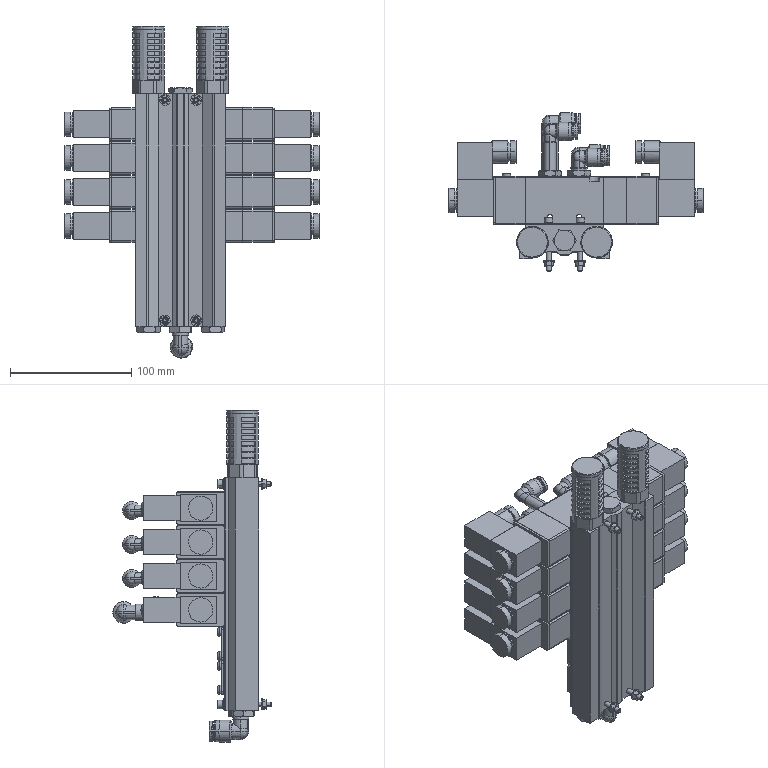Part | SolidWorks | features ReferencePattern 6, LocalLPattern 1 | 41 solids | 2617 faces | box 209.8 x 130.6 x 274 mm | volume 1263291 mm3 | plane 1030 | cylinder 921 | cone 490 | torus 161 | sphere 15 | commonest cylinder face diameters 2.4 x104 23 x96 15 x44 4 x40 4.3 x32 4.5 x32